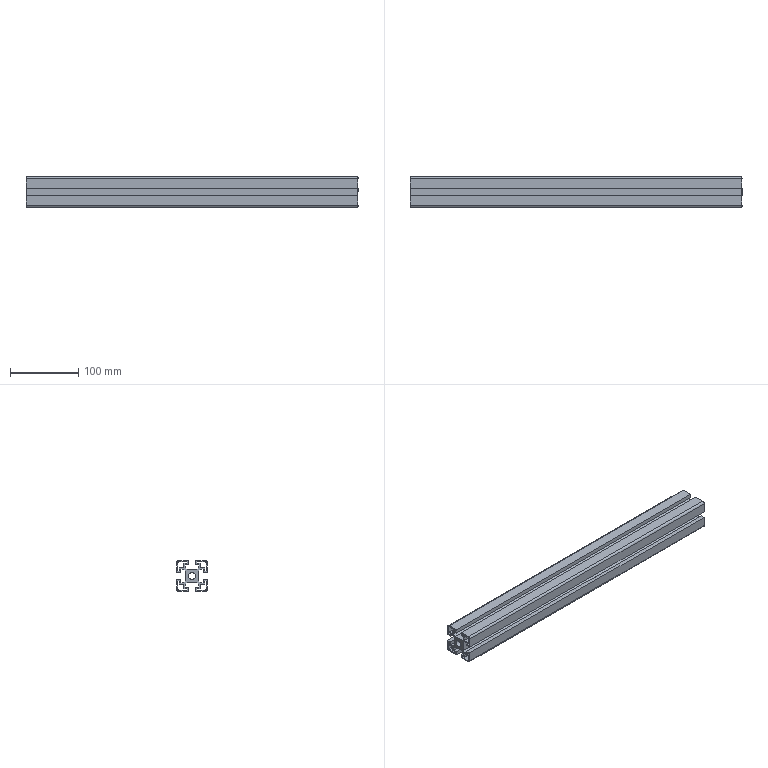Part | STEP file | bosch_3842990520_4ea8orsd7ktxgd8l9ys4v93ta | 1 solid | 87 faces | box 485 x 45 x 45 mm | volume 396605 mm3 | plane 78 | cylinder 9 | commonest cylinder face diameters 2 x4 6 x4 10 x1